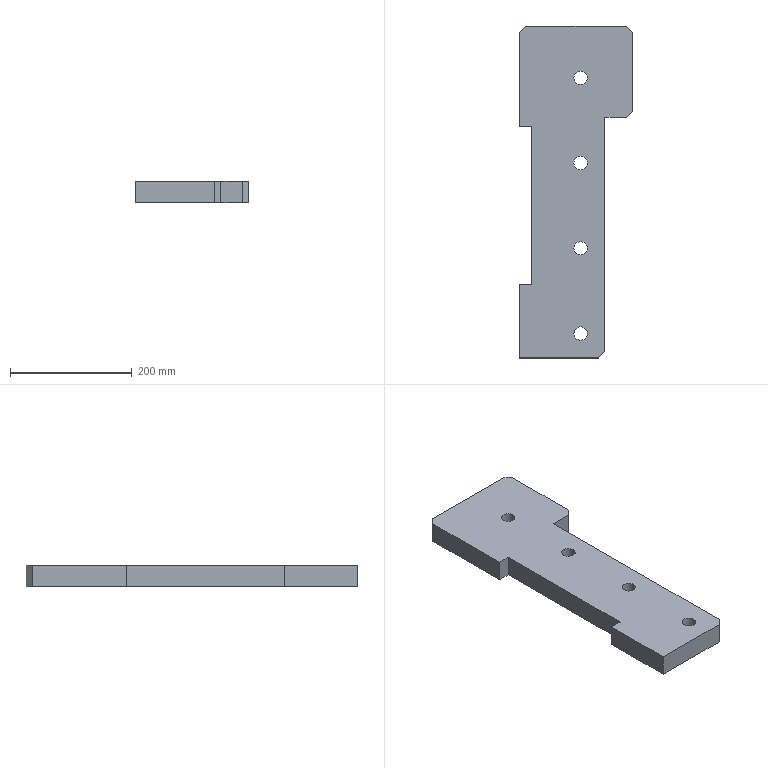Part | SolidWorks | features Chamfer 1, Extrusion 1, ICE 1 | 1 solid | 24 faces | box 185 x 545 x 35 mm | volume 2664531 mm3 | plane 16 | cylinder 8 | commonest cylinder face diameters 22 x8
STEP:
#1=CARTESIAN_POINT('',(89.,-85.,0.));
#2=VERTEX_POINT('',#1);
#3=CARTESIAN_POINT('',(111.,-85.,0.));
#4=VERTEX_POINT('',#3);
#5=CARTESIAN_POINT('',(100.,-85.,0.));
#6=DIRECTION('',(0.,0.,1.));
#7=DIRECTION('',(1.,0.,0.));
#8=AXIS2_PLACEMENT_3D('',#5,#6,#7);
#9=CIRCLE('',#8,11.);
#10=EDGE_CURVE('',#2,#4,#9,.T.);
#11=ORIENTED_EDGE('',*,*,#10,.F.);
#12=CARTESIAN_POINT('',(89.,-85.,35.));
#13=VERTEX_POINT('',#12);
#14=CARTESIAN_POINT('',(89.,-85.,0.));
#15=DIRECTION('',(0.,0.,1.));
#16=VECTOR('',#15,1000.);
#17=LINE('',#14,#16);
#18=EDGE_CURVE('',#2,#13,#17,.T.);
#19=ORIENTED_EDGE('',*,*,#18,.T.);
#20=CARTESIAN_POINT('',(111.,-85.,35.));
#21=VERTEX_POINT('',#20);
#22=CARTESIAN_POINT('',(100.,-85.,35.));
#23=DIRECTION('',(0.,0.,1.));
#24=DIRECTION('',(1.,0.,0.));
#25=AXIS2_PLACEMENT_3D('',#22,#23,#24);
#26=CIRCLE('',#25,11.);
#27=EDGE_CURVE('',#13,#21,#26,.T.);
#28=ORIENTED_EDGE('',*,*,#27,.T.);
#29=CARTESIAN_POINT('',(111.,-85.,0.));
#30=DIRECTION('',(0.,0.,1.));
#31=VECTOR('',#30,1000.);
#32=LINE('',#29,#31);
#33=EDGE_CURVE('',#4,#21,#32,.T.);
#34=ORIENTED_EDGE('',*,*,#33,.F.);
#35=EDGE_LOOP('',(#11,#19,#28,#34));
#36=FACE_OUTER_BOUND('',#35,.T.);
#37=CARTESIAN_POINT('',(100.,-85.,0.));
#38=DIRECTION('',(0.,0.,1.));
#39=DIRECTION('',(1.,0.,0.));
#40=AXIS2_PLACEMENT_3D('',#37,#38,#39);
#41=CYLINDRICAL_SURFACE('',#40,11.);
#42=ADVANCED_FACE('',(#36),#41,.F.);
#43=CARTESIAN_POINT('',(89.,-225.,0.));
#44=VERTEX_POINT('',#43);
#45=CARTESIAN_POINT('',(111.,-225.,0.));
#46=VERTEX_POINT('',#45);
#47=CARTESIAN_POINT('',(100.,-225.,0.));
#48=DIRECTION('',(0.,0.,1.));
#49=DIRECTION('',(1.,0.,0.));
#50=AXIS2_PLACEMENT_3D('',#47,#48,#49);
#51=CIRCLE('',#50,11.);
#52=EDGE_CURVE('',#44,#46,#51,.T.);
#53=ORIENTED_EDGE('',*,*,#52,.F.);
#54=CARTESIAN_POINT('',(89.,-225.,35.));
#55=VERTEX_POINT('',#54);
#56=CARTESIAN_POINT('',(89.,-225.,0.));
#57=DIRECTION('',(0.,0.,1.));
#58=VECTOR('',#57,1000.);
#59=LINE('',#56,#58);
#60=EDGE_CURVE('',#44,#55,#59,.T.);
#61=ORIENTED_EDGE('',*,*,#60,.T.);
#62=CARTESIAN_POINT('',(111.,-225.,35.));
#63=VERTEX_POINT('',#62);
#64=CARTESIAN_POINT('',(100.,-225.,35.));
#65=DIRECTION('',(0.,0.,1.));
#66=DIRECTION('',(1.,0.,0.));
#67=AXIS2_PLACEMENT_3D('',#64,#65,#66);
#68=CIRCLE('',#67,11.);
#69=EDGE_CURVE('',#55,#63,#68,.T.);
#70=ORIENTED_EDGE('',*,*,#69,.T.);
#71=CARTESIAN_POINT('',(111.,-225.,0.));
#72=DIRECTION('',(0.,0.,1.));
#73=VECTOR('',#72,1000.);
#74=LINE('',#71,#73);
#75=EDGE_CURVE('',#46,#63,#74,.T.);
#76=ORIENTED_EDGE('',*,*,#75,.F.);
#77=EDGE_LOOP('',(#53,#61,#70,#76));
#78=FACE_OUTER_BOUND('',#77,.T.);
#79=CARTESIAN_POINT('',(100.,-225.,0.));
#80=DIRECTION('',(0.,0.,1.));
#81=DIRECTION('',(1.,0.,0.));
#82=AXIS2_PLACEMENT_3D('',#79,#80,#81);
#83=CYLINDRICAL_SURFACE('',#82,11.);
#84=ADVANCED_FACE('',(#78),#83,.F.);
#85=CARTESIAN_POINT('',(89.,-365.,0.));
#86=VERTEX_POINT('',#85);
#87=CARTESIAN_POINT('',(111.,-365.,0.));
#88=VERTEX_POINT('',#87);
#89=CARTESIAN_POINT('',(100.,-365.,0.));
#90=DIRECTION('',(0.,0.,1.));
#91=DIRECTION('',(1.,0.,0.));
#92=AXIS2_PLACEMENT_3D('',#89,#90,#91);
#93=CIRCLE('',#92,11.);
#94=EDGE_CURVE('',#86,#88,#93,.T.);
#95=ORIENTED_EDGE('',*,*,#94,.F.);
#96=CARTESIAN_POINT('',(89.,-365.,35.));
#97=VERTEX_POINT('',#96);
#98=CARTESIAN_POINT('',(89.,-365.,0.));
#99=DIRECTION('',(0.,0.,1.));
#100=VECTOR('',#99,1000.);
#101=LINE('',#98,#100);
#102=EDGE_CURVE('',#86,#97,#101,.T.);
#103=ORIENTED_EDGE('',*,*,#102,.T.);
#104=CARTESIAN_POINT('',(111.,-365.,35.));
#105=VERTEX_POINT('',#104);
#106=CARTESIAN_POINT('',(100.,-365.,35.));
#107=DIRECTION('',(0.,0.,1.));
#108=DIRECTION('',(1.,0.,0.));
#109=AXIS2_PLACEMENT_3D('',#106,#107,#108);
#110=CIRCLE('',#109,11.);
#111=EDGE_CURVE('',#97,#105,#110,.T.);
#112=ORIENTED_EDGE('',*,*,#111,.T.);
#113=CARTESIAN_POINT('',(111.,-365.,0.));
#114=DIRECTION('',(0.,0.,1.));
#115=VECTOR('',#114,1000.);
#116=LINE('',#113,#115);
#117=EDGE_CURVE('',#88,#105,#116,.T.);
#118=ORIENTED_EDGE('',*,*,#117,.F.);
#119=EDGE_LOOP('',(#95,#103,#112,#118));
#120=FACE_OUTER_BOUND('',#119,.T.);
#121=CARTESIAN_POINT('',(100.,-365.,0.));
#122=DIRECTION('',(0.,0.,1.));
#123=DIRECTION('',(1.,0.,0.));
#124=AXIS2_PLACEMENT_3D('',#121,#122,#123);
#125=CYLINDRICAL_SURFACE('',#124,11.);
#126=ADVANCED_FACE('',(#120),#125,.F.);
#127=CARTESIAN_POINT('',(89.,-505.,0.));
#128=VERTEX_POINT('',#127);
#129=CARTESIAN_POINT('',(111.,-505.,0.));
#130=VERTEX_POINT('',#129);
#131=CARTESIAN_POINT('',(100.,-505.,0.));
#132=DIRECTION('',(0.,0.,1.));
#133=DIRECTION('',(1.,0.,0.));
#134=AXIS2_PLACEMENT_3D('',#131,#132,#133);
#135=CIRCLE('',#134,11.);
#136=EDGE_CURVE('',#128,#130,#135,.T.);
#137=ORIENTED_EDGE('',*,*,#136,.F.);
#138=CARTESIAN_POINT('',(89.,-505.,35.));
#139=VERTEX_POINT('',#138);
#140=CARTESIAN_POINT('',(89.,-505.,0.));
#141=DIRECTION('',(0.,0.,1.));
#142=VECTOR('',#141,1000.);
#143=LINE('',#140,#142);
#144=EDGE_CURVE('',#128,#139,#143,.T.);
#145=ORIENTED_EDGE('',*,*,#144,.T.);
#146=CARTESIAN_POINT('',(111.,-505.,35.));
#147=VERTEX_POINT('',#146);
#148=CARTESIAN_POINT('',(100.,-505.,35.));
#149=DIRECTION('',(0.,0.,1.));
#150=DIRECTION('',(1.,0.,0.));
#151=AXIS2_PLACEMENT_3D('',#148,#149,#150);
#152=CIRCLE('',#151,11.);
#153=EDGE_CURVE('',#139,#147,#152,.T.);
#154=ORIENTED_EDGE('',*,*,#153,.T.);
#155=CARTESIAN_POINT('',(111.,-505.,0.));
#156=DIRECTION('',(0.,0.,1.));
#157=VECTOR('',#156,1000.);
#158=LINE('',#155,#157);
#159=EDGE_CURVE('',#130,#147,#158,.T.);
#160=ORIENTED_EDGE('',*,*,#159,.F.);
#161=EDGE_LOOP('',(#137,#145,#154,#160));
#162=FACE_OUTER_BOUND('',#161,.T.);
#163=CARTESIAN_POINT('',(100.,-505.,0.));
#164=DIRECTION('',(0.,0.,1.));
#165=DIRECTION('',(1.,0.,0.));
#166=AXIS2_PLACEMENT_3D('',#163,#164,#165);
#167=CYLINDRICAL_SURFACE('',#166,11.);
#168=ADVANCED_FACE('',(#162),#167,.F.);
#169=CARTESIAN_POINT('',(140.,-150.,0.));
#170=VERTEX_POINT('',#169);
#171=CARTESIAN_POINT('',(175.,-150.,0.));
#172=VERTEX_POINT('',#171);
#173=CARTESIAN_POINT('',(185.,-150.,0.));
#174=DIRECTION('',(1.,0.,0.));
#175=VECTOR('',#174,1000.);
#176=LINE('',#173,#175);
#177=EDGE_CURVE('',#170,#172,#176,.T.);
#178=ORIENTED_EDGE('',*,*,#177,.T.);
#179=CARTESIAN_POINT('',(175.,-150.,35.));
#180=VERTEX_POINT('',#179);
#181=CARTESIAN_POINT('',(175.,-150.,35.));
#182=DIRECTION('',(0.,0.,1.));
#183=VECTOR('',#182,1000.);
#184=LINE('',#181,#183);
#185=EDGE_CURVE('',#172,#180,#184,.T.);
#186=ORIENTED_EDGE('',*,*,#185,.T.);
#187=CARTESIAN_POINT('',(140.,-150.,35.));
#188=VERTEX_POINT('',#187);
#189=CARTESIAN_POINT('',(185.,-150.,35.));
#190=DIRECTION('',(1.,0.,0.));
#191=VECTOR('',#190,1000.);
#192=LINE('',#189,#191);
#193=EDGE_CURVE('',#188,#180,#192,.T.);
#194=ORIENTED_EDGE('',*,*,#193,.F.);
#195=CARTESIAN_POINT('',(140.,-150.,35.));
#196=DIRECTION('',(0.,0.,-1.));
#197=VECTOR('',#196,1000.);
#198=LINE('',#195,#197);
#199=EDGE_CURVE('',#188,#170,#198,.T.);
#200=ORIENTED_EDGE('',*,*,#199,.T.);
#201=EDGE_LOOP('',(#178,#186,#194,#200));
#202=FACE_OUTER_BOUND('',#201,.T.);
#203=CARTESIAN_POINT('',(185.,-150.,35.));
#204=DIRECTION('',(0.,1.,0.));
#205=DIRECTION('',(0.,0.,1.));
#206=AXIS2_PLACEMENT_3D('',#203,#204,#205);
#207=PLANE('',#206);
#208=ADVANCED_FACE('',(#202),#207,.F.);
#209=CARTESIAN_POINT('',(185.,-140.,35.));
#210=VERTEX_POINT('',#209);
#211=CARTESIAN_POINT('',(185.,-10.,35.));
#212=VERTEX_POINT('',#211);
#213=CARTESIAN_POINT('',(185.,-150.,35.));
#214=DIRECTION('',(0.,1.,0.));
#215=VECTOR('',#214,1000.);
#216=LINE('',#213,#215);
#217=EDGE_CURVE('',#210,#212,#216,.T.);
#218=ORIENTED_EDGE('',*,*,#217,.F.);
#219=CARTESIAN_POINT('',(185.,-140.,0.));
#220=VERTEX_POINT('',#219);
#221=CARTESIAN_POINT('',(185.,-140.,35.));
#222=DIRECTION('',(0.,0.,-1.));
#223=VECTOR('',#222,1000.);
#224=LINE('',#221,#223);
#225=EDGE_CURVE('',#210,#220,#224,.T.);
#226=ORIENTED_EDGE('',*,*,#225,.T.);
#227=CARTESIAN_POINT('',(185.,-10.,0.));
#228=VERTEX_POINT('',#227);
#229=CARTESIAN_POINT('',(185.,-150.,0.));
#230=DIRECTION('',(0.,1.,0.));
#231=VECTOR('',#230,1000.);
#232=LINE('',#229,#231);
#233=EDGE_CURVE('',#220,#228,#232,.T.);
#234=ORIENTED_EDGE('',*,*,#233,.T.);
#235=CARTESIAN_POINT('',(185.,-10.,35.));
#236=DIRECTION('',(0.,0.,1.));
#237=VECTOR('',#236,1000.);
#238=LINE('',#235,#237);
#239=EDGE_CURVE('',#228,#212,#238,.T.);
#240=ORIENTED_EDGE('',*,*,#239,.T.);
#241=EDGE_LOOP('',(#218,#226,#234,#240));
#242=FACE_OUTER_BOUND('',#241,.T.);
#243=CARTESIAN_POINT('',(185.,-150.,35.));
#244=DIRECTION('',(-1.,0.,0.));
#245=DIRECTION('',(0.,0.,1.));
#246=AXIS2_PLACEMENT_3D('',#243,#244,#245);
#247=PLANE('',#246);
#248=ADVANCED_FACE('',(#242),#247,.F.);
#249=CARTESIAN_POINT('',(175.,0.,0.));
#250=VERTEX_POINT('',#249);
#251=CARTESIAN_POINT('',(10.,0.,0.));
#252=VERTEX_POINT('',#251);
#253=CARTESIAN_POINT('',(185.,0.,0.));
#254=DIRECTION('',(-1.,0.,0.));
#255=VECTOR('',#254,1000.);
#256=LINE('',#253,#255);
#257=EDGE_CURVE('',#250,#252,#256,.T.);
#258=ORIENTED_EDGE('',*,*,#257,.T.);
#259=CARTESIAN_POINT('',(10.,0.,35.));
#260=VERTEX_POINT('',#259);
#261=CARTESIAN_POINT('',(10.,0.,35.));
#262=DIRECTION('',(0.,0.,1.));
#263=VECTOR('',#262,1000.);
#264=LINE('',#261,#263);
#265=EDGE_CURVE('',#252,#260,#264,.T.);
#266=ORIENTED_EDGE('',*,*,#265,.T.);
#267=CARTESIAN_POINT('',(175.,0.,35.));
#268=VERTEX_POINT('',#267);
#269=CARTESIAN_POINT('',(185.,0.,35.));
#270=DIRECTION('',(-1.,0.,0.));
#271=VECTOR('',#270,1000.);
#272=LINE('',#269,#271);
#273=EDGE_CURVE('',#268,#260,#272,.T.);
#274=ORIENTED_EDGE('',*,*,#273,.F.);
#275=CARTESIAN_POINT('',(175.,0.,35.));
#276=DIRECTION('',(0.,0.,-1.));
#277=VECTOR('',#276,1000.);
#278=LINE('',#275,#277);
#279=EDGE_CURVE('',#268,#250,#278,.T.);
#280=ORIENTED_EDGE('',*,*,#279,.T.);
#281=EDGE_LOOP('',(#258,#266,#274,#280));
#282=FACE_OUTER_BOUND('',#281,.T.);
#283=CARTESIAN_POINT('',(185.,0.,35.));
#284=DIRECTION('',(0.,-1.,0.));
#285=DIRECTION('',(0.,0.,-1.));
#286=AXIS2_PLACEMENT_3D('',#283,#284,#285);
#287=PLANE('',#286);
#288=ADVANCED_FACE('',(#282),#287,.F.);
#289=CARTESIAN_POINT('',(0.,-10.,35.));
#290=VERTEX_POINT('',#289);
#291=CARTESIAN_POINT('',(0.,-165.,35.));
#292=VERTEX_POINT('',#291);
#293=CARTESIAN_POINT('',(0.,0.,35.));
#294=DIRECTION('',(0.,-1.,0.));
#295=VECTOR('',#294,1000.);
#296=LINE('',#293,#295);
#297=EDGE_CURVE('',#290,#292,#296,.T.);
#298=ORIENTED_EDGE('',*,*,#297,.F.);
#299=CARTESIAN_POINT('',(0.,-10.,0.));
#300=VERTEX_POINT('',#299);
#301=CARTESIAN_POINT('',(0.,-10.,35.));
#302=DIRECTION('',(0.,0.,-1.));
#303=VECTOR('',#302,1000.);
#304=LINE('',#301,#303);
#305=EDGE_CURVE('',#290,#300,#304,.T.);
#306=ORIENTED_EDGE('',*,*,#305,.T.);
#307=CARTESIAN_POINT('',(0.,-165.,0.));
#308=VERTEX_POINT('',#307);
#309=CARTESIAN_POINT('',(0.,0.,0.));
#310=DIRECTION('',(0.,-1.,0.));
#311=VECTOR('',#310,1000.);
#312=LINE('',#309,#311);
#313=EDGE_CURVE('',#300,#308,#312,.T.);
#314=ORIENTED_EDGE('',*,*,#313,.T.);
#315=CARTESIAN_POINT('',(0.,-165.,35.));
#316=DIRECTION('',(0.,0.,-1.));
#317=VECTOR('',#316,1000.);
#318=LINE('',#315,#317);
#319=EDGE_CURVE('',#292,#308,#318,.T.);
#320=ORIENTED_EDGE('',*,*,#319,.F.);
#321=EDGE_LOOP('',(#298,#306,#314,#320));
#322=FACE_OUTER_BOUND('',#321,.T.);
#323=CARTESIAN_POINT('',(0.,0.,35.));
#324=DIRECTION('',(1.,0.,0.));
#325=DIRECTION('',(0.,1.,0.));
#326=AXIS2_PLACEMENT_3D('',#323,#324,#325);
#327=PLANE('',#326);
#328=ADVANCED_FACE('',(#322),#327,.F.);
#329=CARTESIAN_POINT('',(20.,-165.,0.));
#330=VERTEX_POINT('',#329);
#331=CARTESIAN_POINT('',(0.,-165.,0.));
#332=DIRECTION('',(1.,0.,0.));
#333=VECTOR('',#332,1000.);
#334=LINE('',#331,#333);
#335=EDGE_CURVE('',#308,#330,#334,.T.);
#336=ORIENTED_EDGE('',*,*,#335,.T.);
#337=CARTESIAN_POINT('',(20.,-165.,35.));
#338=VERTEX_POINT('',#337);
#339=CARTESIAN_POINT('',(20.,-165.,35.));
#340=DIRECTION('',(0.,0.,-1.));
#341=VECTOR('',#340,1000.);
#342=LINE('',#339,#341);
#343=EDGE_CURVE('',#338,#330,#342,.T.);
#344=ORIENTED_EDGE('',*,*,#343,.F.);
#345=CARTESIAN_POINT('',(0.,-165.,35.));
#346=DIRECTION('',(1.,0.,0.));
#347=VECTOR('',#346,1000.);
#348=LINE('',#345,#347);
#349=EDGE_CURVE('',#292,#338,#348,.T.);
#350=ORIENTED_EDGE('',*,*,#349,.F.);
#351=ORIENTED_EDGE('',*,*,#319,.T.);
#352=EDGE_LOOP('',(#336,#344,#350,#351));
#353=FACE_OUTER_BOUND('',#352,.T.);
#354=CARTESIAN_POINT('',(0.,-165.,35.));
#355=DIRECTION('',(0.,1.,0.));
#356=DIRECTION('',(0.,0.,1.));
#357=AXIS2_PLACEMENT_3D('',#354,#355,#356);
#358=PLANE('',#357);
#359=ADVANCED_FACE('',(#353),#358,.F.);
#360=CARTESIAN_POINT('',(20.,-425.,0.));
#361=VERTEX_POINT('',#360);
#362=CARTESIAN_POINT('',(20.,-425.,0.));
#363=DIRECTION('',(0.,-1.,0.));
#364=VECTOR('',#363,1000.);
#365=LINE('',#362,#364);
#366=EDGE_CURVE('',#330,#361,#365,.T.);
#367=ORIENTED_EDGE('',*,*,#366,.T.);
#368=CARTESIAN_POINT('',(20.,-425.,35.));
#369=VERTEX_POINT('',#368);
#370=CARTESIAN_POINT('',(20.,-425.,35.));
#371=DIRECTION('',(0.,0.,-1.));
#372=VECTOR('',#371,1000.);
#373=LINE('',#370,#372);
#374=EDGE_CURVE('',#369,#361,#373,.T.);
#375=ORIENTED_EDGE('',*,*,#374,.F.);
#376=CARTESIAN_POINT('',(20.,-425.,35.));
#377=DIRECTION('',(0.,-1.,0.));
#378=VECTOR('',#377,1000.);
#379=LINE('',#376,#378);
#380=EDGE_CURVE('',#338,#369,#379,.T.);
#381=ORIENTED_EDGE('',*,*,#380,.F.);
#382=ORIENTED_EDGE('',*,*,#343,.T.);
#383=EDGE_LOOP('',(#367,#375,#381,#382));
#384=FACE_OUTER_BOUND('',#383,.T.);
#385=CARTESIAN_POINT('',(20.,-425.,35.));
#386=DIRECTION('',(1.,0.,0.));
#387=DIRECTION('',(0.,0.,-1.));
#388=AXIS2_PLACEMENT_3D('',#385,#386,#387);
#389=PLANE('',#388);
#390=ADVANCED_FACE('',(#384),#389,.F.);
#391=CARTESIAN_POINT('',(0.,-425.,0.));
#392=VERTEX_POINT('',#391);
#393=CARTESIAN_POINT('',(0.,-425.,0.));
#394=DIRECTION('',(-1.,0.,0.));
#395=VECTOR('',#394,1000.);
#396=LINE('',#393,#395);
#397=EDGE_CURVE('',#361,#392,#396,.T.);
#398=ORIENTED_EDGE('',*,*,#397,.T.);
#399=CARTESIAN_POINT('',(0.,-425.,35.));
#400=VERTEX_POINT('',#399);
#401=CARTESIAN_POINT('',(0.,-425.,35.));
#402=DIRECTION('',(0.,0.,-1.));
#403=VECTOR('',#402,1000.);
#404=LINE('',#401,#403);
#405=EDGE_CURVE('',#400,#392,#404,.T.);
#406=ORIENTED_EDGE('',*,*,#405,.F.);
#407=CARTESIAN_POINT('',(0.,-425.,35.));
#408=DIRECTION('',(-1.,0.,0.));
#409=VECTOR('',#408,1000.);
#410=LINE('',#407,#409);
#411=EDGE_CURVE('',#369,#400,#410,.T.);
#412=ORIENTED_EDGE('',*,*,#411,.F.);
#413=ORIENTED_EDGE('',*,*,#374,.T.);
#414=EDGE_LOOP('',(#398,#406,#412,#413));
#415=FACE_OUTER_BOUND('',#414,.T.);
#416=CARTESIAN_POINT('',(0.,-425.,35.));
#417=DIRECTION('',(0.,-1.,0.));
#418=DIRECTION('',(0.,0.,-1.));
#419=AXIS2_PLACEMENT_3D('',#416,#417,#418);
#420=PLANE('',#419);
#421=ADVANCED_FACE('',(#415),#420,.F.);
#422=CARTESIAN_POINT('',(0.,-545.,0.));
#423=VERTEX_POINT('',#422);
#424=CARTESIAN_POINT('',(0.,-545.,0.));
#425=DIRECTION('',(0.,-1.,0.));
#426=VECTOR('',#425,1000.);
#427=LINE('',#424,#426);
#428=EDGE_CURVE('',#392,#423,#427,.T.);
#429=ORIENTED_EDGE('',*,*,#428,.T.);
#430=CARTESIAN_POINT('',(0.,-545.,35.));
#431=VERTEX_POINT('',#430);
#432=CARTESIAN_POINT('',(0.,-545.,35.));
#433=DIRECTION('',(0.,0.,-1.));
#434=VECTOR('',#433,1000.);
#435=LINE('',#432,#434);
#436=EDGE_CURVE('',#431,#423,#435,.T.);
#437=ORIENTED_EDGE('',*,*,#436,.F.);
#438=CARTESIAN_POINT('',(0.,-545.,35.));
#439=DIRECTION('',(0.,-1.,0.));
#440=VECTOR('',#439,1000.);
#441=LINE('',#438,#440);
#442=EDGE_CURVE('',#400,#431,#441,.T.);
#443=ORIENTED_EDGE('',*,*,#442,.F.);
#444=ORIENTED_EDGE('',*,*,#405,.T.);
#445=EDGE_LOOP('',(#429,#437,#443,#444));
#446=FACE_OUTER_BOUND('',#445,.T.);
#447=CARTESIAN_POINT('',(0.,-545.,35.));
#448=DIRECTION('',(1.,0.,0.));
#449=DIRECTION('',(0.,0.,-1.));
#450=AXIS2_PLACEMENT_3D('',#447,#448,#449);
#451=PLANE('',#450);
#452=ADVANCED_FACE('',(#446),#451,.F.);
#453=CARTESIAN_POINT('',(130.,-545.,0.));
#454=VERTEX_POINT('',#453);
#455=CARTESIAN_POINT('',(140.,-545.,0.));
#456=DIRECTION('',(1.,0.,0.));
#457=VECTOR('',#456,1000.);
#458=LINE('',#455,#457);
#459=EDGE_CURVE('',#423,#454,#458,.T.);
#460=ORIENTED_EDGE('',*,*,#459,.T.);
#461=CARTESIAN_POINT('',(130.,-545.,35.));
#462=VERTEX_POINT('',#461);
#463=CARTESIAN_POINT('',(130.,-545.,35.));
#464=DIRECTION('',(0.,0.,1.));
#465=VECTOR('',#464,1000.);
#466=LINE('',#463,#465);
#467=EDGE_CURVE('',#454,#462,#466,.T.);
#468=ORIENTED_EDGE('',*,*,#467,.T.);
#469=CARTESIAN_POINT('',(140.,-545.,35.));
#470=DIRECTION('',(1.,0.,0.));
#471=VECTOR('',#470,1000.);
#472=LINE('',#469,#471);
#473=EDGE_CURVE('',#431,#462,#472,.T.);
#474=ORIENTED_EDGE('',*,*,#473,.F.);
#475=ORIENTED_EDGE('',*,*,#436,.T.);
#476=EDGE_LOOP('',(#460,#468,#474,#475));
#477=FACE_OUTER_BOUND('',#476,.T.);
#478=CARTESIAN_POINT('',(140.,-545.,35.));
#479=DIRECTION('',(0.,1.,0.));
#480=DIRECTION('',(0.,0.,1.));
#481=AXIS2_PLACEMENT_3D('',#478,#479,#480);
#482=PLANE('',#481);
#483=ADVANCED_FACE('',(#477),#482,.F.);
#484=CARTESIAN_POINT('',(140.,-535.,35.));
#485=VERTEX_POINT('',#484);
#486=CARTESIAN_POINT('',(140.,-150.,35.));
#487=DIRECTION('',(0.,1.,0.));
#488=VECTOR('',#487,1000.);
#489=LINE('',#486,#488);
#490=EDGE_CURVE('',#485,#188,#489,.T.);
#491=ORIENTED_EDGE('',*,*,#490,.F.);
#492=CARTESIAN_POINT('',(140.,-535.,0.));
#493=VERTEX_POINT('',#492);
#494=CARTESIAN_POINT('',(140.,-535.,35.));
#495=DIRECTION('',(0.,0.,-1.));
#496=VECTOR('',#495,1000.);
#497=LINE('',#494,#496);
#498=EDGE_CURVE('',#485,#493,#497,.T.);
#499=ORIENTED_EDGE('',*,*,#498,.T.);
#500=CARTESIAN_POINT('',(140.,-150.,0.));
#501=DIRECTION('',(0.,1.,0.));
#502=VECTOR('',#501,1000.);
#503=LINE('',#500,#502);
#504=EDGE_CURVE('',#493,#170,#503,.T.);
#505=ORIENTED_EDGE('',*,*,#504,.T.);
#506=ORIENTED_EDGE('',*,*,#199,.F.);
#507=EDGE_LOOP('',(#491,#499,#505,#506));
#508=FACE_OUTER_BOUND('',#507,.T.);
#509=CARTESIAN_POINT('',(140.,-150.,35.));
#510=DIRECTION('',(-1.,0.,0.));
#511=DIRECTION('',(0.,-1.,0.));
#512=AXIS2_PLACEMENT_3D('',#509,#510,#511);
#513=PLANE('',#512);
#514=ADVANCED_FACE('',(#508),#513,.F.);
#515=CARTESIAN_POINT('',(100.,-85.,35.));
#516=DIRECTION('',(0.,0.,1.));
#517=DIRECTION('',(1.,0.,0.));
#518=AXIS2_PLACEMENT_3D('',#515,#516,#517);
#519=CIRCLE('',#518,11.);
#520=EDGE_CURVE('',#21,#13,#519,.T.);
#521=ORIENTED_EDGE('',*,*,#520,.F.);
#522=ORIENTED_EDGE('',*,*,#27,.F.);
#523=EDGE_LOOP('',(#521,#522));
#524=FACE_BOUND('',#523,.T.);
#525=CARTESIAN_POINT('',(100.,-225.,35.));
#526=DIRECTION('',(0.,0.,1.));
#527=DIRECTION('',(1.,0.,0.));
#528=AXIS2_PLACEMENT_3D('',#525,#526,#527);
#529=CIRCLE('',#528,11.);
#530=EDGE_CURVE('',#63,#55,#529,.T.);
#531=ORIENTED_EDGE('',*,*,#530,.F.);
#532=ORIENTED_EDGE('',*,*,#69,.F.);
#533=EDGE_LOOP('',(#531,#532));
#534=FACE_BOUND('',#533,.T.);
#535=CARTESIAN_POINT('',(100.,-365.,35.));
#536=DIRECTION('',(0.,0.,1.));
#537=DIRECTION('',(1.,0.,0.));
#538=AXIS2_PLACEMENT_3D('',#535,#536,#537);
#539=CIRCLE('',#538,11.);
#540=EDGE_CURVE('',#105,#97,#539,.T.);
#541=ORIENTED_EDGE('',*,*,#540,.F.);
#542=ORIENTED_EDGE('',*,*,#111,.F.);
#543=EDGE_LOOP('',(#541,#542));
#544=FACE_BOUND('',#543,.T.);
#545=CARTESIAN_POINT('',(100.,-505.,35.));
#546=DIRECTION('',(0.,0.,1.));
#547=DIRECTION('',(1.,0.,0.));
#548=AXIS2_PLACEMENT_3D('',#545,#546,#547);
#549=CIRCLE('',#548,11.);
#550=EDGE_CURVE('',#147,#139,#549,.T.);
#551=ORIENTED_EDGE('',*,*,#550,.F.);
#552=ORIENTED_EDGE('',*,*,#153,.F.);
#553=EDGE_LOOP('',(#551,#552));
#554=FACE_BOUND('',#553,.T.);
#555=ORIENTED_EDGE('',*,*,#473,.T.);
#556=CARTESIAN_POINT('',(337.5,-337.5,35.));
#557=DIRECTION('',(0.7071,0.7071,0.));
#558=VECTOR('',#557,1000.);
#559=LINE('',#556,#558);
#560=EDGE_CURVE('',#462,#485,#559,.T.);
#561=ORIENTED_EDGE('',*,*,#560,.T.);
#562=ORIENTED_EDGE('',*,*,#490,.T.);
#563=ORIENTED_EDGE('',*,*,#193,.T.);
#564=CARTESIAN_POINT('',(162.5,-162.5,35.));
#565=DIRECTION('',(0.7071,0.7071,0.));
#566=VECTOR('',#565,1000.);
#567=LINE('',#564,#566);
#568=EDGE_CURVE('',#180,#210,#567,.T.);
#569=ORIENTED_EDGE('',*,*,#568,.T.);
#570=ORIENTED_EDGE('',*,*,#217,.T.);
#571=CARTESIAN_POINT('',(87.5,87.5,35.));
#572=DIRECTION('',(-0.7071,0.7071,0.));
#573=VECTOR('',#572,1000.);
#574=LINE('',#571,#573);
#575=EDGE_CURVE('',#212,#268,#574,.T.);
#576=ORIENTED_EDGE('',*,*,#575,.T.);
#577=ORIENTED_EDGE('',*,*,#273,.T.);
#578=CARTESIAN_POINT('',(5.,-5.,35.));
#579=DIRECTION('',(-0.7071,-0.7071,0.));
#580=VECTOR('',#579,1000.);
#581=LINE('',#578,#580);
#582=EDGE_CURVE('',#260,#290,#581,.T.);
#583=ORIENTED_EDGE('',*,*,#582,.T.);
#584=ORIENTED_EDGE('',*,*,#297,.T.);
#585=ORIENTED_EDGE('',*,*,#349,.T.);
#586=ORIENTED_EDGE('',*,*,#380,.T.);
#587=ORIENTED_EDGE('',*,*,#411,.T.);
#588=ORIENTED_EDGE('',*,*,#442,.T.);
#589=EDGE_LOOP('',(#555,#561,#562,#563,#569,#570,#576,#577,#583,#584,#585,#586,#587,#588));
#590=FACE_OUTER_BOUND('',#589,.T.);
#591=CARTESIAN_POINT('',(0.,0.,35.));
#592=DIRECTION('',(0.,0.,1.));
#593=DIRECTION('',(1.,0.,0.));
#594=AXIS2_PLACEMENT_3D('',#591,#592,#593);
#595=PLANE('',#594);
#596=ADVANCED_FACE('',(#524,#534,#544,#554,#590),#595,.T.);
#597=CARTESIAN_POINT('',(100.,-85.,0.));
#598=DIRECTION('',(0.,0.,1.));
#599=DIRECTION('',(1.,0.,0.));
#600=AXIS2_PLACEMENT_3D('',#597,#598,#599);
#601=CIRCLE('',#600,11.);
#602=EDGE_CURVE('',#4,#2,#601,.T.);
#603=ORIENTED_EDGE('',*,*,#602,.T.);
#604=ORIENTED_EDGE('',*,*,#10,.T.);
#605=EDGE_LOOP('',(#603,#604));
#606=FACE_BOUND('',#605,.T.);
#607=CARTESIAN_POINT('',(100.,-225.,0.));
#608=DIRECTION('',(0.,0.,1.));
#609=DIRECTION('',(1.,0.,0.));
#610=AXIS2_PLACEMENT_3D('',#607,#608,#609);
#611=CIRCLE('',#610,11.);
#612=EDGE_CURVE('',#46,#44,#611,.T.);
#613=ORIENTED_EDGE('',*,*,#612,.T.);
#614=ORIENTED_EDGE('',*,*,#52,.T.);
#615=EDGE_LOOP('',(#613,#614));
#616=FACE_BOUND('',#615,.T.);
#617=CARTESIAN_POINT('',(100.,-365.,0.));
#618=DIRECTION('',(0.,0.,1.));
#619=DIRECTION('',(1.,0.,0.));
#620=AXIS2_PLACEMENT_3D('',#617,#618,#619);
#621=CIRCLE('',#620,11.);
#622=EDGE_CURVE('',#88,#86,#621,.T.);
#623=ORIENTED_EDGE('',*,*,#622,.T.);
#624=ORIENTED_EDGE('',*,*,#94,.T.);
#625=EDGE_LOOP('',(#623,#624));
#626=FACE_BOUND('',#625,.T.);
#627=CARTESIAN_POINT('',(100.,-505.,0.));
#628=DIRECTION('',(0.,0.,1.));
#629=DIRECTION('',(1.,0.,0.));
#630=AXIS2_PLACEMENT_3D('',#627,#628,#629);
#631=CIRCLE('',#630,11.);
#632=EDGE_CURVE('',#130,#128,#631,.T.);
#633=ORIENTED_EDGE('',*,*,#632,.T.);
#634=ORIENTED_EDGE('',*,*,#136,.T.);
#635=EDGE_LOOP('',(#633,#634));
#636=FACE_BOUND('',#635,.T.);
#637=ORIENTED_EDGE('',*,*,#504,.F.);
#638=CARTESIAN_POINT('',(140.,-535.,0.));
#639=DIRECTION('',(-0.7071,-0.7071,0.));
#640=VECTOR('',#639,1000.);
#641=LINE('',#638,#640);
#642=EDGE_CURVE('',#493,#454,#641,.T.);
#643=ORIENTED_EDGE('',*,*,#642,.T.);
#644=ORIENTED_EDGE('',*,*,#459,.F.);
#645=ORIENTED_EDGE('',*,*,#428,.F.);
#646=ORIENTED_EDGE('',*,*,#397,.F.);
#647=ORIENTED_EDGE('',*,*,#366,.F.);
#648=ORIENTED_EDGE('',*,*,#335,.F.);
#649=ORIENTED_EDGE('',*,*,#313,.F.);
#650=CARTESIAN_POINT('',(0.,-10.,0.));
#651=DIRECTION('',(0.7071,0.7071,0.));
#652=VECTOR('',#651,1000.);
#653=LINE('',#650,#652);
#654=EDGE_CURVE('',#300,#252,#653,.T.);
#655=ORIENTED_EDGE('',*,*,#654,.T.);
#656=ORIENTED_EDGE('',*,*,#257,.F.);
#657=CARTESIAN_POINT('',(175.,0.,0.));
#658=DIRECTION('',(0.7071,-0.7071,0.));
#659=VECTOR('',#658,1000.);
#660=LINE('',#657,#659);
#661=EDGE_CURVE('',#250,#228,#660,.T.);
#662=ORIENTED_EDGE('',*,*,#661,.T.);
#663=ORIENTED_EDGE('',*,*,#233,.F.);
#664=CARTESIAN_POINT('',(185.,-140.,0.));
#665=DIRECTION('',(-0.7071,-0.7071,0.));
#666=VECTOR('',#665,1000.);
#667=LINE('',#664,#666);
#668=EDGE_CURVE('',#220,#172,#667,.T.);
#669=ORIENTED_EDGE('',*,*,#668,.T.);
#670=ORIENTED_EDGE('',*,*,#177,.F.);
#671=EDGE_LOOP('',(#637,#643,#644,#645,#646,#647,#648,#649,#655,#656,#662,#663,#669,#670));
#672=FACE_OUTER_BOUND('',#671,.T.);
#673=CARTESIAN_POINT('',(0.,0.,0.));
#674=DIRECTION('',(0.,0.,1.));
#675=DIRECTION('',(1.,0.,0.));
#676=AXIS2_PLACEMENT_3D('',#673,#674,#675);
#677=PLANE('',#676);
#678=ADVANCED_FACE('',(#606,#616,#626,#636,#672),#677,.F.);
#679=ORIENTED_EDGE('',*,*,#560,.F.);
#680=ORIENTED_EDGE('',*,*,#467,.F.);
#681=ORIENTED_EDGE('',*,*,#642,.F.);
#682=ORIENTED_EDGE('',*,*,#498,.F.);
#683=EDGE_LOOP('',(#679,#680,#681,#682));
#684=FACE_OUTER_BOUND('',#683,.T.);
#685=CARTESIAN_POINT('',(140.,-535.,35.));
#686=DIRECTION('',(-0.7071,0.7071,0.));
#687=DIRECTION('',(0.,0.,-1.));
#688=AXIS2_PLACEMENT_3D('',#685,#686,#687);
#689=PLANE('',#688);
#690=ADVANCED_FACE('',(#684),#689,.F.);
#691=ORIENTED_EDGE('',*,*,#568,.F.);
#692=ORIENTED_EDGE('',*,*,#185,.F.);
#693=ORIENTED_EDGE('',*,*,#668,.F.);
#694=ORIENTED_EDGE('',*,*,#225,.F.);
#695=EDGE_LOOP('',(#691,#692,#693,#694));
#696=FACE_OUTER_BOUND('',#695,.T.);
#697=CARTESIAN_POINT('',(185.,-140.,35.));
#698=DIRECTION('',(-0.7071,0.7071,0.));
#699=DIRECTION('',(0.,0.,-1.));
#700=AXIS2_PLACEMENT_3D('',#697,#698,#699);
#701=PLANE('',#700);
#702=ADVANCED_FACE('',(#696),#701,.F.);
#703=ORIENTED_EDGE('',*,*,#582,.F.);
#704=ORIENTED_EDGE('',*,*,#265,.F.);
#705=ORIENTED_EDGE('',*,*,#654,.F.);
#706=ORIENTED_EDGE('',*,*,#305,.F.);
#707=EDGE_LOOP('',(#703,#704,#705,#706));
#708=FACE_OUTER_BOUND('',#707,.T.);
#709=CARTESIAN_POINT('',(0.,-10.,35.));
#710=DIRECTION('',(0.7071,-0.7071,0.));
#711=DIRECTION('',(0.,0.,-1.));
#712=AXIS2_PLACEMENT_3D('',#709,#710,#711);
#713=PLANE('',#712);
#714=ADVANCED_FACE('',(#708),#713,.F.);
#715=ORIENTED_EDGE('',*,*,#575,.F.);
#716=ORIENTED_EDGE('',*,*,#239,.F.);
#717=ORIENTED_EDGE('',*,*,#661,.F.);
#718=ORIENTED_EDGE('',*,*,#279,.F.);
#719=EDGE_LOOP('',(#715,#716,#717,#718));
#720=FACE_OUTER_BOUND('',#719,.T.);
#721=CARTESIAN_POINT('',(175.,0.,35.));
#722=DIRECTION('',(-0.7071,-0.7071,0.));
#723=DIRECTION('',(0.,0.,-1.));
#724=AXIS2_PLACEMENT_3D('',#721,#722,#723);
#725=PLANE('',#724);
#726=ADVANCED_FACE('',(#720),#725,.F.);
#727=ORIENTED_EDGE('',*,*,#144,.F.);
#728=ORIENTED_EDGE('',*,*,#632,.F.);
#729=ORIENTED_EDGE('',*,*,#159,.T.);
#730=ORIENTED_EDGE('',*,*,#550,.T.);
#731=EDGE_LOOP('',(#727,#728,#729,#730));
#732=FACE_OUTER_BOUND('',#731,.T.);
#733=CARTESIAN_POINT('',(100.,-505.,0.));
#734=DIRECTION('',(0.,0.,1.));
#735=DIRECTION('',(1.,0.,0.));
#736=AXIS2_PLACEMENT_3D('',#733,#734,#735);
#737=CYLINDRICAL_SURFACE('',#736,11.);
#738=ADVANCED_FACE('',(#732),#737,.F.);
#739=ORIENTED_EDGE('',*,*,#102,.F.);
#740=ORIENTED_EDGE('',*,*,#622,.F.);
#741=ORIENTED_EDGE('',*,*,#117,.T.);
#742=ORIENTED_EDGE('',*,*,#540,.T.);
#743=EDGE_LOOP('',(#739,#740,#741,#742));
#744=FACE_OUTER_BOUND('',#743,.T.);
#745=CARTESIAN_POINT('',(100.,-365.,0.));
#746=DIRECTION('',(0.,0.,1.));
#747=DIRECTION('',(1.,0.,0.));
#748=AXIS2_PLACEMENT_3D('',#745,#746,#747);
#749=CYLINDRICAL_SURFACE('',#748,11.);
#750=ADVANCED_FACE('',(#744),#749,.F.);
#751=ORIENTED_EDGE('',*,*,#60,.F.);
#752=ORIENTED_EDGE('',*,*,#612,.F.);
#753=ORIENTED_EDGE('',*,*,#75,.T.);
#754=ORIENTED_EDGE('',*,*,#530,.T.);
#755=EDGE_LOOP('',(#751,#752,#753,#754));
#756=FACE_OUTER_BOUND('',#755,.T.);
#757=CARTESIAN_POINT('',(100.,-225.,0.));
#758=DIRECTION('',(0.,0.,1.));
#759=DIRECTION('',(1.,0.,0.));
#760=AXIS2_PLACEMENT_3D('',#757,#758,#759);
#761=CYLINDRICAL_SURFACE('',#760,11.);
#762=ADVANCED_FACE('',(#756),#761,.F.);
#763=ORIENTED_EDGE('',*,*,#18,.F.);
#764=ORIENTED_EDGE('',*,*,#602,.F.);
#765=ORIENTED_EDGE('',*,*,#33,.T.);
#766=ORIENTED_EDGE('',*,*,#520,.T.);
#767=EDGE_LOOP('',(#763,#764,#765,#766));
#768=FACE_OUTER_BOUND('',#767,.T.);
#769=CARTESIAN_POINT('',(100.,-85.,0.));
#770=DIRECTION('',(0.,0.,1.));
#771=DIRECTION('',(1.,0.,0.));
#772=AXIS2_PLACEMENT_3D('',#769,#770,#771);
#773=CYLINDRICAL_SURFACE('',#772,11.);
#774=ADVANCED_FACE('',(#768),#773,.F.);
#775=CLOSED_SHELL('',(#42,#84,#126,#168,#208,#248,#288,#328,#359,#390,#421,#452,#483,#514,#596,#678,#690,#702,#714,#726,#738,#750,#762,#774));
#776=MANIFOLD_SOLID_BREP('',#775);
#777=CARTESIAN_POINT('',(0.,0.,0.));
#778=DIRECTION('',(0.,0.,1.));
#779=DIRECTION('',(1.,0.,0.));
#780=AXIS2_PLACEMENT_3D('',#777,#778,#779);
#781=(LENGTH_UNIT()NAMED_UNIT(*)SI_UNIT(.MILLI.,.METRE.));
#782=UNCERTAINTY_MEASURE_WITH_UNIT(LENGTH_MEASURE(0.00001),#781,'','');
#783=(NAMED_UNIT(*)PLANE_ANGLE_UNIT()SI_UNIT($,.RADIAN.));
#784=(NAMED_UNIT(*)SI_UNIT($,.STERADIAN.)SOLID_ANGLE_UNIT());
#785=(GEOMETRIC_REPRESENTATION_CONTEXT(3)GLOBAL_UNCERTAINTY_ASSIGNED_CONTEXT((#782))GLOBAL_UNIT_ASSIGNED_CONTEXT((#781,#783,#784))REPRESENTATION_CONTEXT('',''));
#786=ADVANCED_BREP_SHAPE_REPRESENTATION('',(#776,#780),#785);